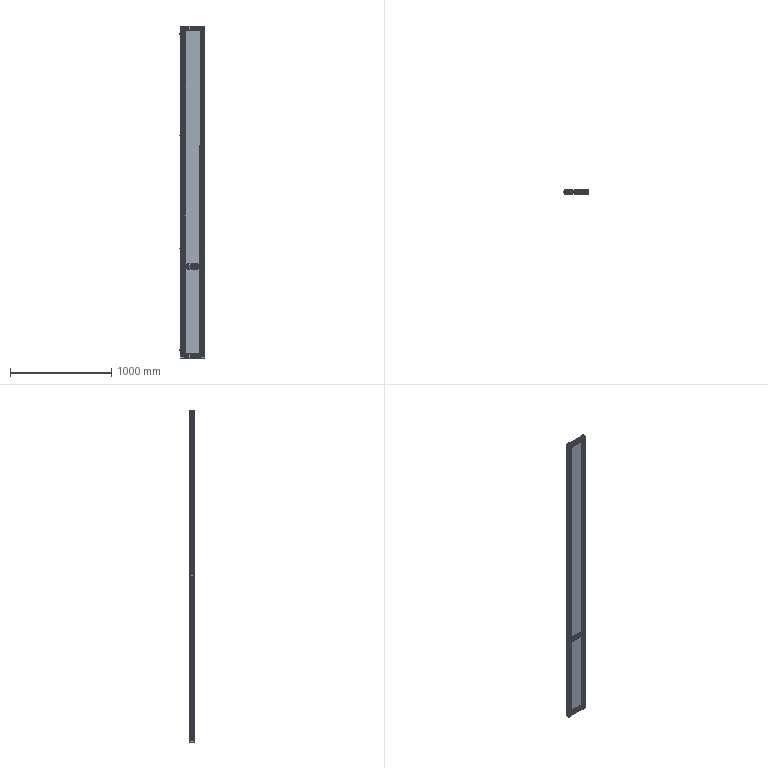Part | SolidWorks | features ReferencePattern 12, LocalLPattern 4 | 67 solids | 3410 faces | volume 7266370 mm3 | plane 2303 | cylinder 935 | cone 140 | spline 32 | commonest cylinder face diameters 0.562 x120 5 x104 6.8 x103 11 x56 2 x54 8 x48